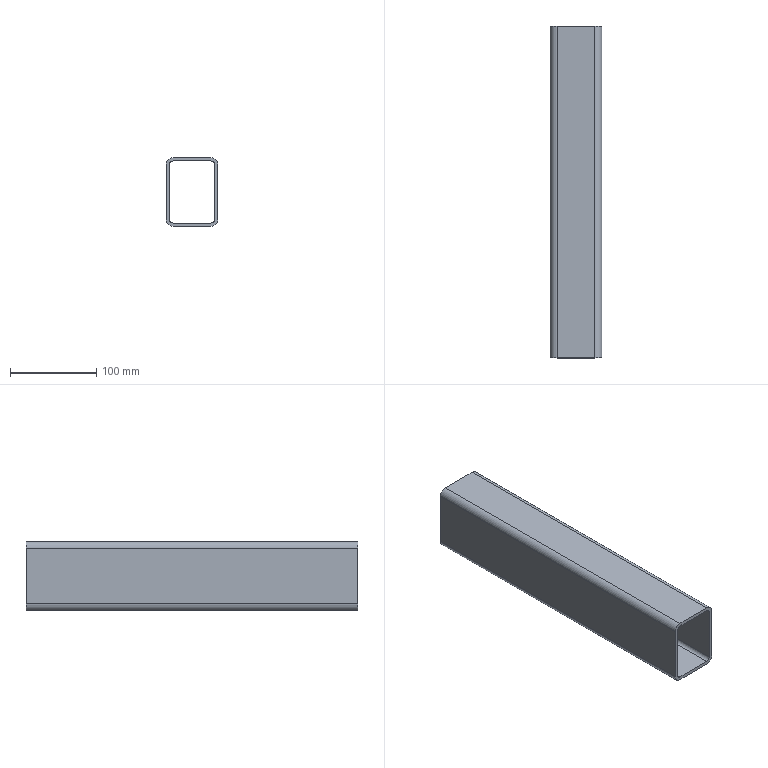Part | SolidWorks | features WeldMemberFeat 1, WeldmentFeature 1 | 1 solid | 18 faces | box 60 x 385 x 80 mm | volume 390697 mm3 | plane 10 | cylinder 8 | commonest cylinder face diameters 8 x4 16 x4
STEP:
#1=CARTESIAN_POINT('',(-30.,0.,32.));
#2=VERTEX_POINT('',#1);
#3=CARTESIAN_POINT('',(-22.,0.,40.));
#4=VERTEX_POINT('',#3);
#5=CARTESIAN_POINT('',(-22.,0.,32.));
#6=DIRECTION('',(0.,1.,0.));
#7=DIRECTION('',(0.,0.,1.));
#8=AXIS2_PLACEMENT_3D('',#5,#6,#7);
#9=CIRCLE('',#8,8.);
#10=EDGE_CURVE('',#2,#4,#9,.T.);
#11=ORIENTED_EDGE('',*,*,#10,.T.);
#12=CARTESIAN_POINT('',(-22.,385.,40.));
#13=VERTEX_POINT('',#12);
#14=CARTESIAN_POINT('',(-22.,385.,40.));
#15=DIRECTION('',(0.,-1.,0.));
#16=VECTOR('',#15,1000.);
#17=LINE('',#14,#16);
#18=EDGE_CURVE('',#13,#4,#17,.T.);
#19=ORIENTED_EDGE('',*,*,#18,.F.);
#20=CARTESIAN_POINT('',(-30.,385.,32.));
#21=VERTEX_POINT('',#20);
#22=CARTESIAN_POINT('',(-22.,385.,32.));
#23=DIRECTION('',(0.,1.,0.));
#24=DIRECTION('',(0.,0.,1.));
#25=AXIS2_PLACEMENT_3D('',#22,#23,#24);
#26=CIRCLE('',#25,8.);
#27=EDGE_CURVE('',#21,#13,#26,.T.);
#28=ORIENTED_EDGE('',*,*,#27,.F.);
#29=CARTESIAN_POINT('',(-30.,385.,32.));
#30=DIRECTION('',(0.,-1.,0.));
#31=VECTOR('',#30,1000.);
#32=LINE('',#29,#31);
#33=EDGE_CURVE('',#21,#2,#32,.T.);
#34=ORIENTED_EDGE('',*,*,#33,.T.);
#35=EDGE_LOOP('',(#11,#19,#28,#34));
#36=FACE_OUTER_BOUND('',#35,.T.);
#37=CARTESIAN_POINT('',(-22.,385.,32.));
#38=DIRECTION('',(0.,-1.,0.));
#39=DIRECTION('',(0.,0.,-1.));
#40=AXIS2_PLACEMENT_3D('',#37,#38,#39);
#41=CYLINDRICAL_SURFACE('',#40,8.);
#42=ADVANCED_FACE('',(#36),#41,.T.);
#43=CARTESIAN_POINT('',(22.,0.,40.));
#44=VERTEX_POINT('',#43);
#45=CARTESIAN_POINT('',(-22.,0.,40.));
#46=DIRECTION('',(1.,0.,0.));
#47=VECTOR('',#46,1000.);
#48=LINE('',#45,#47);
#49=EDGE_CURVE('',#4,#44,#48,.T.);
#50=ORIENTED_EDGE('',*,*,#49,.T.);
#51=CARTESIAN_POINT('',(22.,385.,40.));
#52=VERTEX_POINT('',#51);
#53=CARTESIAN_POINT('',(22.,385.,40.));
#54=DIRECTION('',(0.,-1.,0.));
#55=VECTOR('',#54,1000.);
#56=LINE('',#53,#55);
#57=EDGE_CURVE('',#52,#44,#56,.T.);
#58=ORIENTED_EDGE('',*,*,#57,.F.);
#59=CARTESIAN_POINT('',(-22.,385.,40.));
#60=DIRECTION('',(1.,0.,0.));
#61=VECTOR('',#60,1000.);
#62=LINE('',#59,#61);
#63=EDGE_CURVE('',#13,#52,#62,.T.);
#64=ORIENTED_EDGE('',*,*,#63,.F.);
#65=ORIENTED_EDGE('',*,*,#18,.T.);
#66=EDGE_LOOP('',(#50,#58,#64,#65));
#67=FACE_OUTER_BOUND('',#66,.T.);
#68=CARTESIAN_POINT('',(-22.,385.,40.));
#69=DIRECTION('',(0.,0.,-1.));
#70=DIRECTION('',(-1.,0.,0.));
#71=AXIS2_PLACEMENT_3D('',#68,#69,#70);
#72=PLANE('',#71);
#73=ADVANCED_FACE('',(#67),#72,.F.);
#74=CARTESIAN_POINT('',(30.,0.,32.));
#75=VERTEX_POINT('',#74);
#76=CARTESIAN_POINT('',(22.,0.,32.));
#77=DIRECTION('',(0.,1.,0.));
#78=DIRECTION('',(0.,0.,1.));
#79=AXIS2_PLACEMENT_3D('',#76,#77,#78);
#80=CIRCLE('',#79,8.);
#81=EDGE_CURVE('',#44,#75,#80,.T.);
#82=ORIENTED_EDGE('',*,*,#81,.T.);
#83=CARTESIAN_POINT('',(30.,385.,32.));
#84=VERTEX_POINT('',#83);
#85=CARTESIAN_POINT('',(30.,385.,32.));
#86=DIRECTION('',(0.,-1.,0.));
#87=VECTOR('',#86,1000.);
#88=LINE('',#85,#87);
#89=EDGE_CURVE('',#84,#75,#88,.T.);
#90=ORIENTED_EDGE('',*,*,#89,.F.);
#91=CARTESIAN_POINT('',(22.,385.,32.));
#92=DIRECTION('',(0.,1.,0.));
#93=DIRECTION('',(0.,0.,1.));
#94=AXIS2_PLACEMENT_3D('',#91,#92,#93);
#95=CIRCLE('',#94,8.);
#96=EDGE_CURVE('',#52,#84,#95,.T.);
#97=ORIENTED_EDGE('',*,*,#96,.F.);
#98=ORIENTED_EDGE('',*,*,#57,.T.);
#99=EDGE_LOOP('',(#82,#90,#97,#98));
#100=FACE_OUTER_BOUND('',#99,.T.);
#101=CARTESIAN_POINT('',(22.,385.,32.));
#102=DIRECTION('',(0.,-1.,0.));
#103=DIRECTION('',(0.,0.,-1.));
#104=AXIS2_PLACEMENT_3D('',#101,#102,#103);
#105=CYLINDRICAL_SURFACE('',#104,8.);
#106=ADVANCED_FACE('',(#100),#105,.T.);
#107=CARTESIAN_POINT('',(30.,0.,-32.));
#108=VERTEX_POINT('',#107);
#109=CARTESIAN_POINT('',(30.,0.,-32.));
#110=DIRECTION('',(0.,0.,-1.));
#111=VECTOR('',#110,1000.);
#112=LINE('',#109,#111);
#113=EDGE_CURVE('',#75,#108,#112,.T.);
#114=ORIENTED_EDGE('',*,*,#113,.T.);
#115=CARTESIAN_POINT('',(30.,385.,-32.));
#116=VERTEX_POINT('',#115);
#117=CARTESIAN_POINT('',(30.,385.,-32.));
#118=DIRECTION('',(0.,-1.,0.));
#119=VECTOR('',#118,1000.);
#120=LINE('',#117,#119);
#121=EDGE_CURVE('',#116,#108,#120,.T.);
#122=ORIENTED_EDGE('',*,*,#121,.F.);
#123=CARTESIAN_POINT('',(30.,385.,-32.));
#124=DIRECTION('',(0.,0.,-1.));
#125=VECTOR('',#124,1000.);
#126=LINE('',#123,#125);
#127=EDGE_CURVE('',#84,#116,#126,.T.);
#128=ORIENTED_EDGE('',*,*,#127,.F.);
#129=ORIENTED_EDGE('',*,*,#89,.T.);
#130=EDGE_LOOP('',(#114,#122,#128,#129));
#131=FACE_OUTER_BOUND('',#130,.T.);
#132=CARTESIAN_POINT('',(30.,385.,-32.));
#133=DIRECTION('',(-1.,0.,0.));
#134=DIRECTION('',(0.,0.,1.));
#135=AXIS2_PLACEMENT_3D('',#132,#133,#134);
#136=PLANE('',#135);
#137=ADVANCED_FACE('',(#131),#136,.F.);
#138=CARTESIAN_POINT('',(22.,0.,-40.));
#139=VERTEX_POINT('',#138);
#140=CARTESIAN_POINT('',(22.,0.,-32.));
#141=DIRECTION('',(0.,1.,0.));
#142=DIRECTION('',(0.,0.,1.));
#143=AXIS2_PLACEMENT_3D('',#140,#141,#142);
#144=CIRCLE('',#143,8.);
#145=EDGE_CURVE('',#108,#139,#144,.T.);
#146=ORIENTED_EDGE('',*,*,#145,.T.);
#147=CARTESIAN_POINT('',(22.,385.,-40.));
#148=VERTEX_POINT('',#147);
#149=CARTESIAN_POINT('',(22.,385.,-40.));
#150=DIRECTION('',(0.,-1.,0.));
#151=VECTOR('',#150,1000.);
#152=LINE('',#149,#151);
#153=EDGE_CURVE('',#148,#139,#152,.T.);
#154=ORIENTED_EDGE('',*,*,#153,.F.);
#155=CARTESIAN_POINT('',(22.,385.,-32.));
#156=DIRECTION('',(0.,1.,0.));
#157=DIRECTION('',(0.,0.,1.));
#158=AXIS2_PLACEMENT_3D('',#155,#156,#157);
#159=CIRCLE('',#158,8.);
#160=EDGE_CURVE('',#116,#148,#159,.T.);
#161=ORIENTED_EDGE('',*,*,#160,.F.);
#162=ORIENTED_EDGE('',*,*,#121,.T.);
#163=EDGE_LOOP('',(#146,#154,#161,#162));
#164=FACE_OUTER_BOUND('',#163,.T.);
#165=CARTESIAN_POINT('',(22.,385.,-32.));
#166=DIRECTION('',(0.,-1.,0.));
#167=DIRECTION('',(0.,0.,-1.));
#168=AXIS2_PLACEMENT_3D('',#165,#166,#167);
#169=CYLINDRICAL_SURFACE('',#168,8.);
#170=ADVANCED_FACE('',(#164),#169,.T.);
#171=CARTESIAN_POINT('',(-22.,0.,-40.));
#172=VERTEX_POINT('',#171);
#173=CARTESIAN_POINT('',(22.,0.,-40.));
#174=DIRECTION('',(-1.,0.,0.));
#175=VECTOR('',#174,1000.);
#176=LINE('',#173,#175);
#177=EDGE_CURVE('',#139,#172,#176,.T.);
#178=ORIENTED_EDGE('',*,*,#177,.T.);
#179=CARTESIAN_POINT('',(-22.,385.,-40.));
#180=VERTEX_POINT('',#179);
#181=CARTESIAN_POINT('',(-22.,385.,-40.));
#182=DIRECTION('',(0.,-1.,0.));
#183=VECTOR('',#182,1000.);
#184=LINE('',#181,#183);
#185=EDGE_CURVE('',#180,#172,#184,.T.);
#186=ORIENTED_EDGE('',*,*,#185,.F.);
#187=CARTESIAN_POINT('',(22.,385.,-40.));
#188=DIRECTION('',(-1.,0.,0.));
#189=VECTOR('',#188,1000.);
#190=LINE('',#187,#189);
#191=EDGE_CURVE('',#148,#180,#190,.T.);
#192=ORIENTED_EDGE('',*,*,#191,.F.);
#193=ORIENTED_EDGE('',*,*,#153,.T.);
#194=EDGE_LOOP('',(#178,#186,#192,#193));
#195=FACE_OUTER_BOUND('',#194,.T.);
#196=CARTESIAN_POINT('',(22.,385.,-40.));
#197=DIRECTION('',(0.,0.,1.));
#198=DIRECTION('',(1.,0.,0.));
#199=AXIS2_PLACEMENT_3D('',#196,#197,#198);
#200=PLANE('',#199);
#201=ADVANCED_FACE('',(#195),#200,.F.);
#202=CARTESIAN_POINT('',(-30.,0.,-32.));
#203=VERTEX_POINT('',#202);
#204=CARTESIAN_POINT('',(-22.,0.,-32.));
#205=DIRECTION('',(0.,1.,0.));
#206=DIRECTION('',(0.,0.,1.));
#207=AXIS2_PLACEMENT_3D('',#204,#205,#206);
#208=CIRCLE('',#207,8.);
#209=EDGE_CURVE('',#172,#203,#208,.T.);
#210=ORIENTED_EDGE('',*,*,#209,.T.);
#211=CARTESIAN_POINT('',(-30.,385.,-32.));
#212=VERTEX_POINT('',#211);
#213=CARTESIAN_POINT('',(-30.,385.,-32.));
#214=DIRECTION('',(0.,-1.,0.));
#215=VECTOR('',#214,1000.);
#216=LINE('',#213,#215);
#217=EDGE_CURVE('',#212,#203,#216,.T.);
#218=ORIENTED_EDGE('',*,*,#217,.F.);
#219=CARTESIAN_POINT('',(-22.,385.,-32.));
#220=DIRECTION('',(0.,1.,0.));
#221=DIRECTION('',(0.,0.,1.));
#222=AXIS2_PLACEMENT_3D('',#219,#220,#221);
#223=CIRCLE('',#222,8.);
#224=EDGE_CURVE('',#180,#212,#223,.T.);
#225=ORIENTED_EDGE('',*,*,#224,.F.);
#226=ORIENTED_EDGE('',*,*,#185,.T.);
#227=EDGE_LOOP('',(#210,#218,#225,#226));
#228=FACE_OUTER_BOUND('',#227,.T.);
#229=CARTESIAN_POINT('',(-22.,385.,-32.));
#230=DIRECTION('',(0.,-1.,0.));
#231=DIRECTION('',(0.,0.,-1.));
#232=AXIS2_PLACEMENT_3D('',#229,#230,#231);
#233=CYLINDRICAL_SURFACE('',#232,8.);
#234=ADVANCED_FACE('',(#228),#233,.T.);
#235=CARTESIAN_POINT('',(22.,0.,36.));
#236=VERTEX_POINT('',#235);
#237=CARTESIAN_POINT('',(26.,0.,32.));
#238=VERTEX_POINT('',#237);
#239=CARTESIAN_POINT('',(22.,0.,32.));
#240=DIRECTION('',(0.,1.,0.));
#241=DIRECTION('',(0.,0.,1.));
#242=AXIS2_PLACEMENT_3D('',#239,#240,#241);
#243=CIRCLE('',#242,4.);
#244=EDGE_CURVE('',#236,#238,#243,.T.);
#245=ORIENTED_EDGE('',*,*,#244,.F.);
#246=CARTESIAN_POINT('',(22.,385.,36.));
#247=VERTEX_POINT('',#246);
#248=CARTESIAN_POINT('',(22.,385.,36.));
#249=DIRECTION('',(0.,-1.,0.));
#250=VECTOR('',#249,1000.);
#251=LINE('',#248,#250);
#252=EDGE_CURVE('',#247,#236,#251,.T.);
#253=ORIENTED_EDGE('',*,*,#252,.F.);
#254=CARTESIAN_POINT('',(26.,385.,32.));
#255=VERTEX_POINT('',#254);
#256=CARTESIAN_POINT('',(22.,385.,32.));
#257=DIRECTION('',(0.,1.,0.));
#258=DIRECTION('',(0.,0.,1.));
#259=AXIS2_PLACEMENT_3D('',#256,#257,#258);
#260=CIRCLE('',#259,4.);
#261=EDGE_CURVE('',#247,#255,#260,.T.);
#262=ORIENTED_EDGE('',*,*,#261,.T.);
#263=CARTESIAN_POINT('',(26.,385.,32.));
#264=DIRECTION('',(0.,-1.,0.));
#265=VECTOR('',#264,1000.);
#266=LINE('',#263,#265);
#267=EDGE_CURVE('',#255,#238,#266,.T.);
#268=ORIENTED_EDGE('',*,*,#267,.T.);
#269=EDGE_LOOP('',(#245,#253,#262,#268));
#270=FACE_OUTER_BOUND('',#269,.T.);
#271=CARTESIAN_POINT('',(22.,385.,32.));
#272=DIRECTION('',(0.,-1.,0.));
#273=DIRECTION('',(0.,0.,-1.));
#274=AXIS2_PLACEMENT_3D('',#271,#272,#273);
#275=CYLINDRICAL_SURFACE('',#274,4.);
#276=ADVANCED_FACE('',(#270),#275,.F.);
#277=CARTESIAN_POINT('',(-22.,0.,36.));
#278=VERTEX_POINT('',#277);
#279=CARTESIAN_POINT('',(-22.,0.,36.));
#280=DIRECTION('',(1.,0.,0.));
#281=VECTOR('',#280,1000.);
#282=LINE('',#279,#281);
#283=EDGE_CURVE('',#278,#236,#282,.T.);
#284=ORIENTED_EDGE('',*,*,#283,.F.);
#285=CARTESIAN_POINT('',(-22.,385.,36.));
#286=VERTEX_POINT('',#285);
#287=CARTESIAN_POINT('',(-22.,385.,36.));
#288=DIRECTION('',(0.,-1.,0.));
#289=VECTOR('',#288,1000.);
#290=LINE('',#287,#289);
#291=EDGE_CURVE('',#286,#278,#290,.T.);
#292=ORIENTED_EDGE('',*,*,#291,.F.);
#293=CARTESIAN_POINT('',(-22.,385.,36.));
#294=DIRECTION('',(1.,0.,0.));
#295=VECTOR('',#294,1000.);
#296=LINE('',#293,#295);
#297=EDGE_CURVE('',#286,#247,#296,.T.);
#298=ORIENTED_EDGE('',*,*,#297,.T.);
#299=ORIENTED_EDGE('',*,*,#252,.T.);
#300=EDGE_LOOP('',(#284,#292,#298,#299));
#301=FACE_OUTER_BOUND('',#300,.T.);
#302=CARTESIAN_POINT('',(-22.,385.,36.));
#303=DIRECTION('',(0.,0.,-1.));
#304=DIRECTION('',(-1.,0.,0.));
#305=AXIS2_PLACEMENT_3D('',#302,#303,#304);
#306=PLANE('',#305);
#307=ADVANCED_FACE('',(#301),#306,.T.);
#308=CARTESIAN_POINT('',(-26.,0.,32.));
#309=VERTEX_POINT('',#308);
#310=CARTESIAN_POINT('',(-22.,0.,32.));
#311=DIRECTION('',(0.,1.,0.));
#312=DIRECTION('',(0.,0.,1.));
#313=AXIS2_PLACEMENT_3D('',#310,#311,#312);
#314=CIRCLE('',#313,4.);
#315=EDGE_CURVE('',#309,#278,#314,.T.);
#316=ORIENTED_EDGE('',*,*,#315,.F.);
#317=CARTESIAN_POINT('',(-26.,385.,32.));
#318=VERTEX_POINT('',#317);
#319=CARTESIAN_POINT('',(-26.,385.,32.));
#320=DIRECTION('',(0.,-1.,0.));
#321=VECTOR('',#320,1000.);
#322=LINE('',#319,#321);
#323=EDGE_CURVE('',#318,#309,#322,.T.);
#324=ORIENTED_EDGE('',*,*,#323,.F.);
#325=CARTESIAN_POINT('',(-22.,385.,32.));
#326=DIRECTION('',(0.,1.,0.));
#327=DIRECTION('',(0.,0.,1.));
#328=AXIS2_PLACEMENT_3D('',#325,#326,#327);
#329=CIRCLE('',#328,4.);
#330=EDGE_CURVE('',#318,#286,#329,.T.);
#331=ORIENTED_EDGE('',*,*,#330,.T.);
#332=ORIENTED_EDGE('',*,*,#291,.T.);
#333=EDGE_LOOP('',(#316,#324,#331,#332));
#334=FACE_OUTER_BOUND('',#333,.T.);
#335=CARTESIAN_POINT('',(-22.,385.,32.));
#336=DIRECTION('',(0.,-1.,0.));
#337=DIRECTION('',(0.,0.,-1.));
#338=AXIS2_PLACEMENT_3D('',#335,#336,#337);
#339=CYLINDRICAL_SURFACE('',#338,4.);
#340=ADVANCED_FACE('',(#334),#339,.F.);
#341=CARTESIAN_POINT('',(-26.,0.,-32.));
#342=VERTEX_POINT('',#341);
#343=CARTESIAN_POINT('',(-26.,0.,32.));
#344=DIRECTION('',(0.,0.,1.));
#345=VECTOR('',#344,1000.);
#346=LINE('',#343,#345);
#347=EDGE_CURVE('',#342,#309,#346,.T.);
#348=ORIENTED_EDGE('',*,*,#347,.F.);
#349=CARTESIAN_POINT('',(-26.,385.,-32.));
#350=VERTEX_POINT('',#349);
#351=CARTESIAN_POINT('',(-26.,385.,-32.));
#352=DIRECTION('',(0.,-1.,0.));
#353=VECTOR('',#352,1000.);
#354=LINE('',#351,#353);
#355=EDGE_CURVE('',#350,#342,#354,.T.);
#356=ORIENTED_EDGE('',*,*,#355,.F.);
#357=CARTESIAN_POINT('',(-26.,385.,32.));
#358=DIRECTION('',(0.,0.,1.));
#359=VECTOR('',#358,1000.);
#360=LINE('',#357,#359);
#361=EDGE_CURVE('',#350,#318,#360,.T.);
#362=ORIENTED_EDGE('',*,*,#361,.T.);
#363=ORIENTED_EDGE('',*,*,#323,.T.);
#364=EDGE_LOOP('',(#348,#356,#362,#363));
#365=FACE_OUTER_BOUND('',#364,.T.);
#366=CARTESIAN_POINT('',(-26.,385.,32.));
#367=DIRECTION('',(1.,0.,0.));
#368=DIRECTION('',(0.,0.,-1.));
#369=AXIS2_PLACEMENT_3D('',#366,#367,#368);
#370=PLANE('',#369);
#371=ADVANCED_FACE('',(#365),#370,.T.);
#372=CARTESIAN_POINT('',(-22.,0.,-36.));
#373=VERTEX_POINT('',#372);
#374=CARTESIAN_POINT('',(-22.,0.,-32.));
#375=DIRECTION('',(0.,1.,0.));
#376=DIRECTION('',(0.,0.,1.));
#377=AXIS2_PLACEMENT_3D('',#374,#375,#376);
#378=CIRCLE('',#377,4.);
#379=EDGE_CURVE('',#373,#342,#378,.T.);
#380=ORIENTED_EDGE('',*,*,#379,.F.);
#381=CARTESIAN_POINT('',(-22.,385.,-36.));
#382=VERTEX_POINT('',#381);
#383=CARTESIAN_POINT('',(-22.,385.,-36.));
#384=DIRECTION('',(0.,-1.,0.));
#385=VECTOR('',#384,1000.);
#386=LINE('',#383,#385);
#387=EDGE_CURVE('',#382,#373,#386,.T.);
#388=ORIENTED_EDGE('',*,*,#387,.F.);
#389=CARTESIAN_POINT('',(-22.,385.,-32.));
#390=DIRECTION('',(0.,1.,0.));
#391=DIRECTION('',(0.,0.,1.));
#392=AXIS2_PLACEMENT_3D('',#389,#390,#391);
#393=CIRCLE('',#392,4.);
#394=EDGE_CURVE('',#382,#350,#393,.T.);
#395=ORIENTED_EDGE('',*,*,#394,.T.);
#396=ORIENTED_EDGE('',*,*,#355,.T.);
#397=EDGE_LOOP('',(#380,#388,#395,#396));
#398=FACE_OUTER_BOUND('',#397,.T.);
#399=CARTESIAN_POINT('',(-22.,385.,-32.));
#400=DIRECTION('',(0.,-1.,0.));
#401=DIRECTION('',(0.,0.,-1.));
#402=AXIS2_PLACEMENT_3D('',#399,#400,#401);
#403=CYLINDRICAL_SURFACE('',#402,4.);
#404=ADVANCED_FACE('',(#398),#403,.F.);
#405=CARTESIAN_POINT('',(22.,0.,-36.));
#406=VERTEX_POINT('',#405);
#407=CARTESIAN_POINT('',(22.,0.,-36.));
#408=DIRECTION('',(-1.,0.,0.));
#409=VECTOR('',#408,1000.);
#410=LINE('',#407,#409);
#411=EDGE_CURVE('',#406,#373,#410,.T.);
#412=ORIENTED_EDGE('',*,*,#411,.F.);
#413=CARTESIAN_POINT('',(22.,385.,-36.));
#414=VERTEX_POINT('',#413);
#415=CARTESIAN_POINT('',(22.,385.,-36.));
#416=DIRECTION('',(0.,-1.,0.));
#417=VECTOR('',#416,1000.);
#418=LINE('',#415,#417);
#419=EDGE_CURVE('',#414,#406,#418,.T.);
#420=ORIENTED_EDGE('',*,*,#419,.F.);
#421=CARTESIAN_POINT('',(22.,385.,-36.));
#422=DIRECTION('',(-1.,0.,0.));
#423=VECTOR('',#422,1000.);
#424=LINE('',#421,#423);
#425=EDGE_CURVE('',#414,#382,#424,.T.);
#426=ORIENTED_EDGE('',*,*,#425,.T.);
#427=ORIENTED_EDGE('',*,*,#387,.T.);
#428=EDGE_LOOP('',(#412,#420,#426,#427));
#429=FACE_OUTER_BOUND('',#428,.T.);
#430=CARTESIAN_POINT('',(22.,385.,-36.));
#431=DIRECTION('',(0.,0.,1.));
#432=DIRECTION('',(1.,0.,0.));
#433=AXIS2_PLACEMENT_3D('',#430,#431,#432);
#434=PLANE('',#433);
#435=ADVANCED_FACE('',(#429),#434,.T.);
#436=CARTESIAN_POINT('',(26.,0.,-32.));
#437=VERTEX_POINT('',#436);
#438=CARTESIAN_POINT('',(22.,0.,-32.));
#439=DIRECTION('',(0.,1.,0.));
#440=DIRECTION('',(0.,0.,1.));
#441=AXIS2_PLACEMENT_3D('',#438,#439,#440);
#442=CIRCLE('',#441,4.);
#443=EDGE_CURVE('',#437,#406,#442,.T.);
#444=ORIENTED_EDGE('',*,*,#443,.F.);
#445=CARTESIAN_POINT('',(26.,385.,-32.));
#446=VERTEX_POINT('',#445);
#447=CARTESIAN_POINT('',(26.,385.,-32.));
#448=DIRECTION('',(0.,-1.,0.));
#449=VECTOR('',#448,1000.);
#450=LINE('',#447,#449);
#451=EDGE_CURVE('',#446,#437,#450,.T.);
#452=ORIENTED_EDGE('',*,*,#451,.F.);
#453=CARTESIAN_POINT('',(22.,385.,-32.));
#454=DIRECTION('',(0.,1.,0.));
#455=DIRECTION('',(0.,0.,1.));
#456=AXIS2_PLACEMENT_3D('',#453,#454,#455);
#457=CIRCLE('',#456,4.);
#458=EDGE_CURVE('',#446,#414,#457,.T.);
#459=ORIENTED_EDGE('',*,*,#458,.T.);
#460=ORIENTED_EDGE('',*,*,#419,.T.);
#461=EDGE_LOOP('',(#444,#452,#459,#460));
#462=FACE_OUTER_BOUND('',#461,.T.);
#463=CARTESIAN_POINT('',(22.,385.,-32.));
#464=DIRECTION('',(0.,-1.,0.));
#465=DIRECTION('',(0.,0.,-1.));
#466=AXIS2_PLACEMENT_3D('',#463,#464,#465);
#467=CYLINDRICAL_SURFACE('',#466,4.);
#468=ADVANCED_FACE('',(#462),#467,.F.);
#469=CARTESIAN_POINT('',(26.,0.,-32.));
#470=DIRECTION('',(0.,0.,-1.));
#471=VECTOR('',#470,1000.);
#472=LINE('',#469,#471);
#473=EDGE_CURVE('',#238,#437,#472,.T.);
#474=ORIENTED_EDGE('',*,*,#473,.F.);
#475=ORIENTED_EDGE('',*,*,#267,.F.);
#476=CARTESIAN_POINT('',(26.,385.,-32.));
#477=DIRECTION('',(0.,0.,-1.));
#478=VECTOR('',#477,1000.);
#479=LINE('',#476,#478);
#480=EDGE_CURVE('',#255,#446,#479,.T.);
#481=ORIENTED_EDGE('',*,*,#480,.T.);
#482=ORIENTED_EDGE('',*,*,#451,.T.);
#483=EDGE_LOOP('',(#474,#475,#481,#482));
#484=FACE_OUTER_BOUND('',#483,.T.);
#485=CARTESIAN_POINT('',(26.,385.,-32.));
#486=DIRECTION('',(-1.,0.,0.));
#487=DIRECTION('',(0.,0.,1.));
#488=AXIS2_PLACEMENT_3D('',#485,#486,#487);
#489=PLANE('',#488);
#490=ADVANCED_FACE('',(#484),#489,.T.);
#491=CARTESIAN_POINT('',(-30.,0.,32.));
#492=DIRECTION('',(0.,0.,1.));
#493=VECTOR('',#492,1000.);
#494=LINE('',#491,#493);
#495=EDGE_CURVE('',#203,#2,#494,.T.);
#496=ORIENTED_EDGE('',*,*,#495,.T.);
#497=ORIENTED_EDGE('',*,*,#33,.F.);
#498=CARTESIAN_POINT('',(-30.,385.,32.));
#499=DIRECTION('',(0.,0.,1.));
#500=VECTOR('',#499,1000.);
#501=LINE('',#498,#500);
#502=EDGE_CURVE('',#212,#21,#501,.T.);
#503=ORIENTED_EDGE('',*,*,#502,.F.);
#504=ORIENTED_EDGE('',*,*,#217,.T.);
#505=EDGE_LOOP('',(#496,#497,#503,#504));
#506=FACE_OUTER_BOUND('',#505,.T.);
#507=CARTESIAN_POINT('',(-30.,385.,32.));
#508=DIRECTION('',(1.,0.,0.));
#509=DIRECTION('',(0.,0.,-1.));
#510=AXIS2_PLACEMENT_3D('',#507,#508,#509);
#511=PLANE('',#510);
#512=ADVANCED_FACE('',(#506),#511,.F.);
#513=ORIENTED_EDGE('',*,*,#261,.F.);
#514=ORIENTED_EDGE('',*,*,#297,.F.);
#515=ORIENTED_EDGE('',*,*,#330,.F.);
#516=ORIENTED_EDGE('',*,*,#361,.F.);
#517=ORIENTED_EDGE('',*,*,#394,.F.);
#518=ORIENTED_EDGE('',*,*,#425,.F.);
#519=ORIENTED_EDGE('',*,*,#458,.F.);
#520=ORIENTED_EDGE('',*,*,#480,.F.);
#521=EDGE_LOOP('',(#513,#514,#515,#516,#517,#518,#519,#520));
#522=FACE_BOUND('',#521,.T.);
#523=ORIENTED_EDGE('',*,*,#27,.T.);
#524=ORIENTED_EDGE('',*,*,#63,.T.);
#525=ORIENTED_EDGE('',*,*,#96,.T.);
#526=ORIENTED_EDGE('',*,*,#127,.T.);
#527=ORIENTED_EDGE('',*,*,#160,.T.);
#528=ORIENTED_EDGE('',*,*,#191,.T.);
#529=ORIENTED_EDGE('',*,*,#224,.T.);
#530=ORIENTED_EDGE('',*,*,#502,.T.);
#531=EDGE_LOOP('',(#523,#524,#525,#526,#527,#528,#529,#530));
#532=FACE_OUTER_BOUND('',#531,.T.);
#533=CARTESIAN_POINT('',(-22.,385.,32.));
#534=DIRECTION('',(0.,1.,0.));
#535=DIRECTION('',(0.,0.,1.));
#536=AXIS2_PLACEMENT_3D('',#533,#534,#535);
#537=PLANE('',#536);
#538=ADVANCED_FACE('',(#522,#532),#537,.T.);
#539=ORIENTED_EDGE('',*,*,#244,.T.);
#540=ORIENTED_EDGE('',*,*,#473,.T.);
#541=ORIENTED_EDGE('',*,*,#443,.T.);
#542=ORIENTED_EDGE('',*,*,#411,.T.);
#543=ORIENTED_EDGE('',*,*,#379,.T.);
#544=ORIENTED_EDGE('',*,*,#347,.T.);
#545=ORIENTED_EDGE('',*,*,#315,.T.);
#546=ORIENTED_EDGE('',*,*,#283,.T.);
#547=EDGE_LOOP('',(#539,#540,#541,#542,#543,#544,#545,#546));
#548=FACE_BOUND('',#547,.T.);
#549=ORIENTED_EDGE('',*,*,#10,.F.);
#550=ORIENTED_EDGE('',*,*,#495,.F.);
#551=ORIENTED_EDGE('',*,*,#209,.F.);
#552=ORIENTED_EDGE('',*,*,#177,.F.);
#553=ORIENTED_EDGE('',*,*,#145,.F.);
#554=ORIENTED_EDGE('',*,*,#113,.F.);
#555=ORIENTED_EDGE('',*,*,#81,.F.);
#556=ORIENTED_EDGE('',*,*,#49,.F.);
#557=EDGE_LOOP('',(#549,#550,#551,#552,#553,#554,#555,#556));
#558=FACE_OUTER_BOUND('',#557,.T.);
#559=CARTESIAN_POINT('',(-22.,0.,32.));
#560=DIRECTION('',(0.,1.,0.));
#561=DIRECTION('',(0.,0.,1.));
#562=AXIS2_PLACEMENT_3D('',#559,#560,#561);
#563=PLANE('',#562);
#564=ADVANCED_FACE('',(#548,#558),#563,.F.);
#565=CLOSED_SHELL('',(#42,#73,#106,#137,#170,#201,#234,#276,#307,#340,#371,#404,#435,#468,#490,#512,#538,#564));
#566=MANIFOLD_SOLID_BREP('',#565);
#567=CARTESIAN_POINT('',(0.,0.,0.));
#568=DIRECTION('',(0.,0.,1.));
#569=DIRECTION('',(1.,0.,0.));
#570=AXIS2_PLACEMENT_3D('',#567,#568,#569);
#571=(LENGTH_UNIT()NAMED_UNIT(*)SI_UNIT(.MILLI.,.METRE.));
#572=UNCERTAINTY_MEASURE_WITH_UNIT(LENGTH_MEASURE(0.00001),#571,'','');
#573=(NAMED_UNIT(*)PLANE_ANGLE_UNIT()SI_UNIT($,.RADIAN.));
#574=(NAMED_UNIT(*)SI_UNIT($,.STERADIAN.)SOLID_ANGLE_UNIT());
#575=(GEOMETRIC_REPRESENTATION_CONTEXT(3)GLOBAL_UNCERTAINTY_ASSIGNED_CONTEXT((#572))GLOBAL_UNIT_ASSIGNED_CONTEXT((#571,#573,#574))REPRESENTATION_CONTEXT('',''));
#576=ADVANCED_BREP_SHAPE_REPRESENTATION('',(#566,#570),#575);